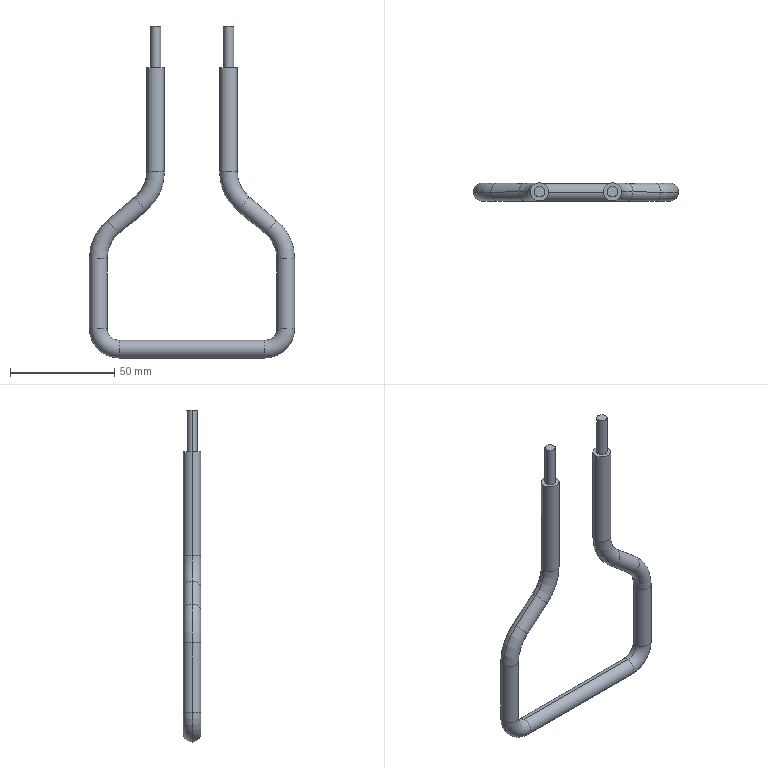Part | STEP file | Heater - SUP.INF | 1 solid | 34 faces | box 98.5 x 8.5 x 159.25 mm | volume 21910 mm3 | cylinder 18 | torus 12 | plane 4 | commonest cylinder face diameters 8.5 x14 5 x4